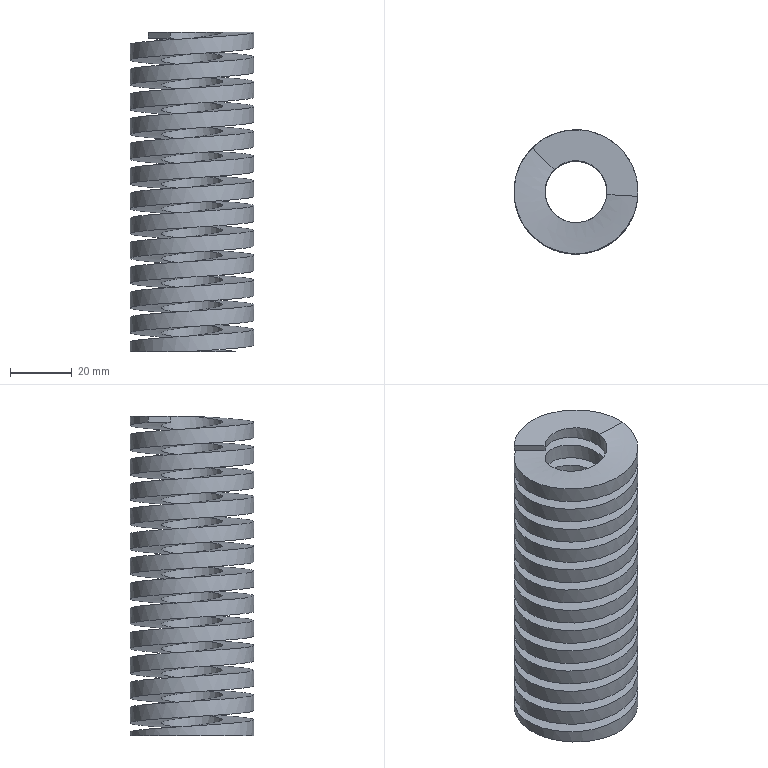Part | STEP file | gslz 2016.10.28-6_id50_x_t | 1 solid | 8 faces | box 40.005 x 40.005 x 103 mm | volume 60665 mm3 | spline 4 | plane 4